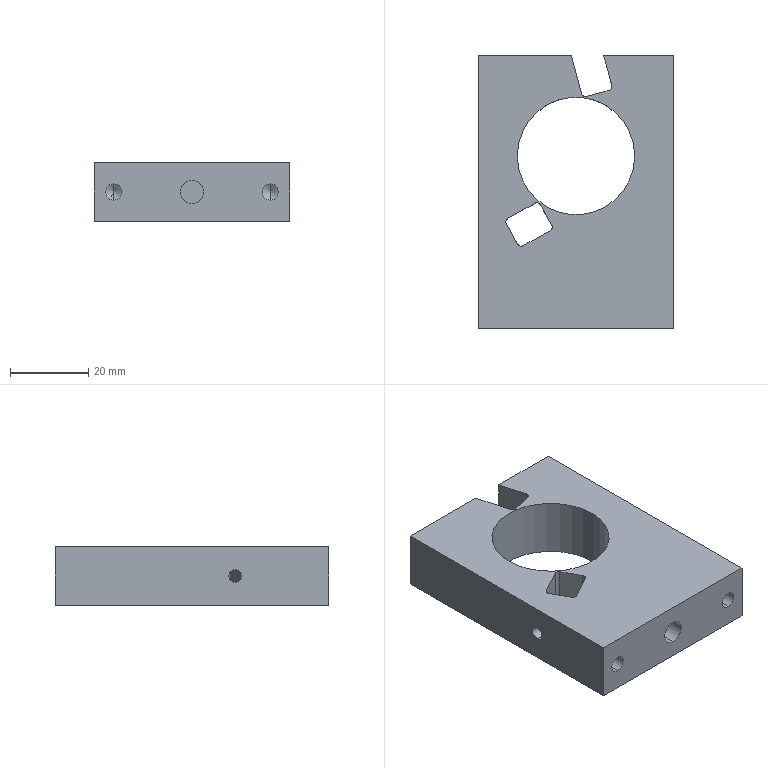Part | STEP file | 04-02-01 left bending mounting plate | 1 solid | 55 faces | box 50 x 70 x 15 mm | volume 38195 mm3 | cylinder 28 | plane 15 | cone 12 | commonest cylinder face diameters 3.3 x12 2 x8 4.2 x4 6 x2 30 x2